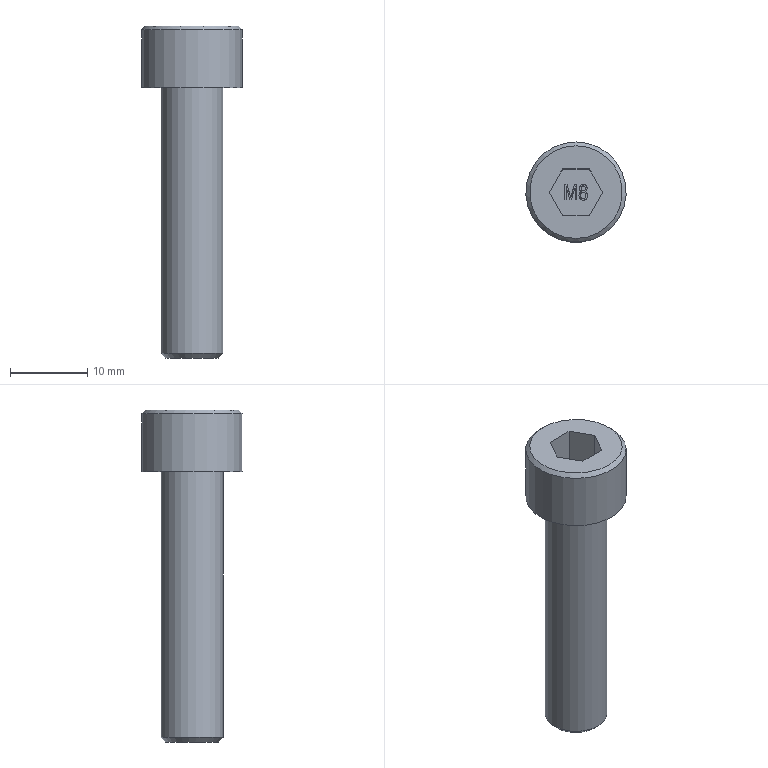Part | STEP file | EM10803500 | 1 solid | 38 faces | box 13 x 13 x 43 mm | volume 2656 mm3 | plane 25 | other 9 | cylinder 2 | cone 2 | commonest cylinder face diameters 8 x1 13 x1